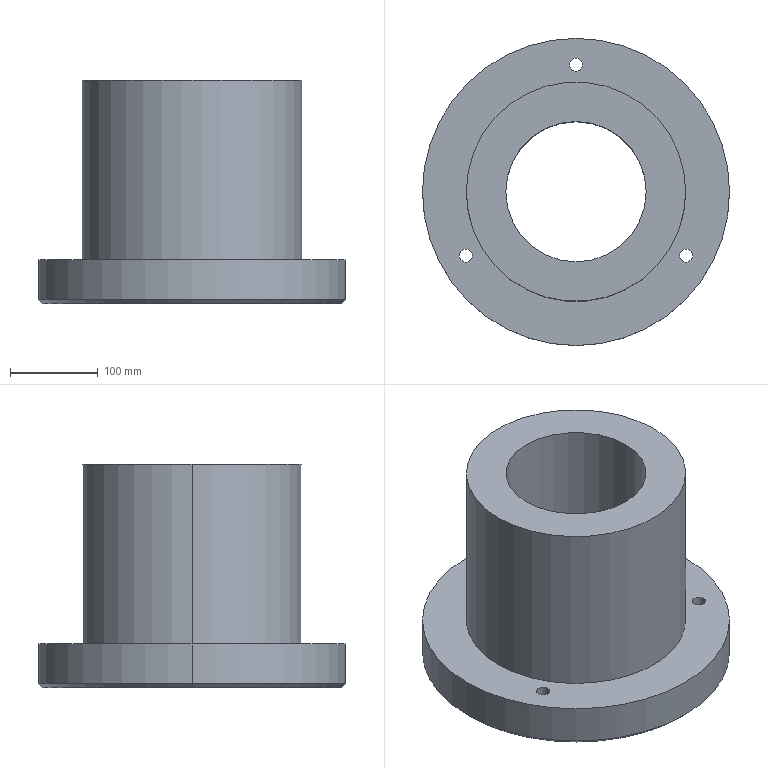Part | SolidWorks | features BaseBody 1 | 1 solid | 26 faces | box 350 x 350 x 255 mm | volume 9479362 mm3 | cylinder 14 | cone 8 | plane 4 | commonest cylinder face diameters 15 x6 160 x2 200 x2 250 x2 350 x2
STEP:
#1=CARTESIAN_POINT('',(345.077,953.249,-619.893));
#2=VERTEX_POINT('',#1);
#3=CARTESIAN_POINT('',(185.077,953.249,-619.893));
#4=VERTEX_POINT('',#3);
#5=CARTESIAN_POINT('',(265.077,953.249,-619.893));
#6=DIRECTION('',(0.,0.,-1.));
#7=DIRECTION('',(-1.,0.,0.));
#8=AXIS2_PLACEMENT_3D('',#5,#6,#7);
#9=CIRCLE('',#8,80.);
#10=EDGE_CURVE('',#2,#4,#9,.T.);
#11=ORIENTED_EDGE('',*,*,#10,.F.);
#12=CARTESIAN_POINT('',(265.077,953.249,-619.893));
#13=DIRECTION('',(0.,0.,-1.));
#14=DIRECTION('',(-1.,0.,0.));
#15=AXIS2_PLACEMENT_3D('',#12,#13,#14);
#16=CIRCLE('',#15,80.);
#17=EDGE_CURVE('',#4,#2,#16,.T.);
#18=ORIENTED_EDGE('',*,*,#17,.F.);
#19=EDGE_LOOP('',(#11,#18));
#20=FACE_BOUND('',#19,.T.);
#21=CARTESIAN_POINT('',(165.077,953.249,-619.893));
#22=VERTEX_POINT('',#21);
#23=CARTESIAN_POINT('',(365.077,953.249,-619.893));
#24=VERTEX_POINT('',#23);
#25=CARTESIAN_POINT('',(265.077,953.249,-619.893));
#26=DIRECTION('',(0.,0.,-1.));
#27=DIRECTION('',(-1.,0.,0.));
#28=AXIS2_PLACEMENT_3D('',#25,#26,#27);
#29=CIRCLE('',#28,100.);
#30=EDGE_CURVE('',#22,#24,#29,.T.);
#31=ORIENTED_EDGE('',*,*,#30,.T.);
#32=CARTESIAN_POINT('',(265.077,953.249,-619.893));
#33=DIRECTION('',(0.,0.,-1.));
#34=DIRECTION('',(-1.,0.,0.));
#35=AXIS2_PLACEMENT_3D('',#32,#33,#34);
#36=CIRCLE('',#35,100.);
#37=EDGE_CURVE('',#24,#22,#36,.T.);
#38=ORIENTED_EDGE('',*,*,#37,.T.);
#39=EDGE_LOOP('',(#31,#38));
#40=FACE_OUTER_BOUND('',#39,.T.);
#41=CARTESIAN_POINT('',(265.077,953.249,-619.893));
#42=DIRECTION('',(0.,0.,-1.));
#43=DIRECTION('',(0.,-1.,0.));
#44=AXIS2_PLACEMENT_3D('',#41,#42,#43);
#45=PLANE('',#44);
#46=ADVANCED_FACE('',(#20,#40),#45,.T.);
#47=CARTESIAN_POINT('',(365.077,953.249,-639.893));
#48=VERTEX_POINT('',#47);
#49=CARTESIAN_POINT('',(365.077,953.249,-619.893));
#50=DIRECTION('',(0.,0.,1.));
#51=VECTOR('',#50,1000.);
#52=LINE('',#49,#51);
#53=EDGE_CURVE('',#48,#24,#52,.T.);
#54=ORIENTED_EDGE('',*,*,#53,.T.);
#55=ORIENTED_EDGE('',*,*,#30,.F.);
#56=CARTESIAN_POINT('',(165.077,953.249,-639.893));
#57=VERTEX_POINT('',#56);
#58=CARTESIAN_POINT('',(165.077,953.249,-619.893));
#59=DIRECTION('',(0.,0.,1.));
#60=VECTOR('',#59,1000.);
#61=LINE('',#58,#60);
#62=EDGE_CURVE('',#57,#22,#61,.T.);
#63=ORIENTED_EDGE('',*,*,#62,.F.);
#64=CARTESIAN_POINT('',(265.077,953.249,-639.893));
#65=DIRECTION('',(0.,0.,-1.));
#66=DIRECTION('',(-1.,0.,0.));
#67=AXIS2_PLACEMENT_3D('',#64,#65,#66);
#68=CIRCLE('',#67,100.);
#69=EDGE_CURVE('',#57,#48,#68,.T.);
#70=ORIENTED_EDGE('',*,*,#69,.T.);
#71=EDGE_LOOP('',(#54,#55,#63,#70));
#72=FACE_OUTER_BOUND('',#71,.T.);
#73=CARTESIAN_POINT('',(265.077,953.249,-619.893));
#74=DIRECTION('',(0.,0.,-1.));
#75=DIRECTION('',(1.,0.,0.));
#76=AXIS2_PLACEMENT_3D('',#73,#74,#75);
#77=CYLINDRICAL_SURFACE('',#76,100.);
#78=ADVANCED_FACE('',(#72),#77,.F.);
#79=CARTESIAN_POINT('',(90.077,953.249,-634.893));
#80=VERTEX_POINT('',#79);
#81=CARTESIAN_POINT('',(95.077,953.249,-639.893));
#82=VERTEX_POINT('',#81);
#83=CARTESIAN_POINT('',(95.077,953.249,-639.893));
#84=DIRECTION('',(0.7071,0.,-0.7071));
#85=VECTOR('',#84,1000.);
#86=LINE('',#83,#85);
#87=EDGE_CURVE('',#80,#82,#86,.T.);
#88=ORIENTED_EDGE('',*,*,#87,.T.);
#89=CARTESIAN_POINT('',(435.077,953.249,-639.893));
#90=VERTEX_POINT('',#89);
#91=CARTESIAN_POINT('',(265.077,953.249,-639.893));
#92=DIRECTION('',(0.,0.,-1.));
#93=DIRECTION('',(-1.,0.,0.));
#94=AXIS2_PLACEMENT_3D('',#91,#92,#93);
#95=CIRCLE('',#94,170.);
#96=EDGE_CURVE('',#90,#82,#95,.T.);
#97=ORIENTED_EDGE('',*,*,#96,.F.);
#98=CARTESIAN_POINT('',(440.077,953.249,-634.893));
#99=VERTEX_POINT('',#98);
#100=CARTESIAN_POINT('',(435.077,953.249,-639.893));
#101=DIRECTION('',(-0.7071,0.,-0.7071));
#102=VECTOR('',#101,1000.);
#103=LINE('',#100,#102);
#104=EDGE_CURVE('',#99,#90,#103,.T.);
#105=ORIENTED_EDGE('',*,*,#104,.F.);
#106=CARTESIAN_POINT('',(265.077,953.249,-634.893));
#107=DIRECTION('',(0.,0.,1.));
#108=DIRECTION('',(-1.,0.,0.));
#109=AXIS2_PLACEMENT_3D('',#106,#107,#108);
#110=CIRCLE('',#109,175.);
#111=EDGE_CURVE('',#80,#99,#110,.T.);
#112=ORIENTED_EDGE('',*,*,#111,.F.);
#113=EDGE_LOOP('',(#88,#97,#105,#112));
#114=FACE_OUTER_BOUND('',#113,.T.);
#115=CARTESIAN_POINT('',(265.077,953.249,-639.893));
#116=DIRECTION('',(0.,0.,1.));
#117=DIRECTION('',(-1.,0.,0.));
#118=AXIS2_PLACEMENT_3D('',#115,#116,#117);
#119=CONICAL_SURFACE('',#118,170.,0.7854);
#120=ADVANCED_FACE('',(#114),#119,.T.);
#121=CARTESIAN_POINT('',(275.577,1098.249,-639.893));
#122=VERTEX_POINT('',#121);
#123=CARTESIAN_POINT('',(272.577,1098.249,-636.893));
#124=VERTEX_POINT('',#123);
#125=CARTESIAN_POINT('',(272.577,1098.249,-636.893));
#126=DIRECTION('',(-0.7071,0.,0.7071));
#127=VECTOR('',#126,1000.);
#128=LINE('',#125,#127);
#129=EDGE_CURVE('',#122,#124,#128,.T.);
#130=ORIENTED_EDGE('',*,*,#129,.T.);
#131=CARTESIAN_POINT('',(257.577,1098.249,-636.893));
#132=VERTEX_POINT('',#131);
#133=CARTESIAN_POINT('',(265.077,1098.249,-636.893));
#134=DIRECTION('',(0.,0.,-1.));
#135=DIRECTION('',(-1.,0.,0.));
#136=AXIS2_PLACEMENT_3D('',#133,#134,#135);
#137=CIRCLE('',#136,7.5);
#138=EDGE_CURVE('',#132,#124,#137,.T.);
#139=ORIENTED_EDGE('',*,*,#138,.F.);
#140=CARTESIAN_POINT('',(254.577,1098.249,-639.893));
#141=VERTEX_POINT('',#140);
#142=CARTESIAN_POINT('',(257.577,1098.249,-636.893));
#143=DIRECTION('',(0.7071,0.,0.7071));
#144=VECTOR('',#143,1000.);
#145=LINE('',#142,#144);
#146=EDGE_CURVE('',#141,#132,#145,.T.);
#147=ORIENTED_EDGE('',*,*,#146,.F.);
#148=CARTESIAN_POINT('',(265.077,1098.249,-639.893));
#149=DIRECTION('',(0.,0.,1.));
#150=DIRECTION('',(-1.,0.,0.));
#151=AXIS2_PLACEMENT_3D('',#148,#149,#150);
#152=CIRCLE('',#151,10.5);
#153=EDGE_CURVE('',#122,#141,#152,.T.);
#154=ORIENTED_EDGE('',*,*,#153,.F.);
#155=EDGE_LOOP('',(#130,#139,#147,#154));
#156=FACE_OUTER_BOUND('',#155,.T.);
#157=CARTESIAN_POINT('',(265.077,1098.249,-636.893));
#158=DIRECTION('',(0.,0.,-1.));
#159=DIRECTION('',(1.,0.,0.));
#160=AXIS2_PLACEMENT_3D('',#157,#158,#159);
#161=CONICAL_SURFACE('',#160,7.5,0.7854);
#162=ADVANCED_FACE('',(#156),#161,.F.);
#163=CARTESIAN_POINT('',(401.151,880.749,-639.893));
#164=VERTEX_POINT('',#163);
#165=CARTESIAN_POINT('',(398.151,880.749,-636.893));
#166=VERTEX_POINT('',#165);
#167=CARTESIAN_POINT('',(398.151,880.749,-636.893));
#168=DIRECTION('',(-0.7071,0.,0.7071));
#169=VECTOR('',#168,1000.);
#170=LINE('',#167,#169);
#171=EDGE_CURVE('',#164,#166,#170,.T.);
#172=ORIENTED_EDGE('',*,*,#171,.T.);
#173=CARTESIAN_POINT('',(383.151,880.749,-636.893));
#174=VERTEX_POINT('',#173);
#175=CARTESIAN_POINT('',(390.651,880.749,-636.893));
#176=DIRECTION('',(0.,0.,-1.));
#177=DIRECTION('',(-1.,0.,0.));
#178=AXIS2_PLACEMENT_3D('',#175,#176,#177);
#179=CIRCLE('',#178,7.5);
#180=EDGE_CURVE('',#174,#166,#179,.T.);
#181=ORIENTED_EDGE('',*,*,#180,.F.);
#182=CARTESIAN_POINT('',(380.151,880.749,-639.893));
#183=VERTEX_POINT('',#182);
#184=CARTESIAN_POINT('',(383.151,880.749,-636.893));
#185=DIRECTION('',(0.7071,0.,0.7071));
#186=VECTOR('',#185,1000.);
#187=LINE('',#184,#186);
#188=EDGE_CURVE('',#183,#174,#187,.T.);
#189=ORIENTED_EDGE('',*,*,#188,.F.);
#190=CARTESIAN_POINT('',(390.651,880.749,-639.893));
#191=DIRECTION('',(0.,0.,1.));
#192=DIRECTION('',(-1.,0.,0.));
#193=AXIS2_PLACEMENT_3D('',#190,#191,#192);
#194=CIRCLE('',#193,10.5);
#195=EDGE_CURVE('',#164,#183,#194,.T.);
#196=ORIENTED_EDGE('',*,*,#195,.F.);
#197=EDGE_LOOP('',(#172,#181,#189,#196));
#198=FACE_OUTER_BOUND('',#197,.T.);
#199=CARTESIAN_POINT('',(390.651,880.749,-636.893));
#200=DIRECTION('',(0.,0.,-1.));
#201=DIRECTION('',(1.,0.,0.));
#202=AXIS2_PLACEMENT_3D('',#199,#200,#201);
#203=CONICAL_SURFACE('',#202,7.5,0.7854);
#204=ADVANCED_FACE('',(#198),#203,.F.);
#205=CARTESIAN_POINT('',(150.003,880.749,-639.893));
#206=VERTEX_POINT('',#205);
#207=CARTESIAN_POINT('',(147.003,880.749,-636.893));
#208=VERTEX_POINT('',#207);
#209=CARTESIAN_POINT('',(147.003,880.749,-636.893));
#210=DIRECTION('',(-0.7071,0.,0.7071));
#211=VECTOR('',#210,1000.);
#212=LINE('',#209,#211);
#213=EDGE_CURVE('',#206,#208,#212,.T.);
#214=ORIENTED_EDGE('',*,*,#213,.T.);
#215=CARTESIAN_POINT('',(132.003,880.749,-636.893));
#216=VERTEX_POINT('',#215);
#217=CARTESIAN_POINT('',(139.503,880.749,-636.893));
#218=DIRECTION('',(0.,0.,-1.));
#219=DIRECTION('',(-1.,0.,0.));
#220=AXIS2_PLACEMENT_3D('',#217,#218,#219);
#221=CIRCLE('',#220,7.5);
#222=EDGE_CURVE('',#216,#208,#221,.T.);
#223=ORIENTED_EDGE('',*,*,#222,.F.);
#224=CARTESIAN_POINT('',(129.003,880.749,-639.893));
#225=VERTEX_POINT('',#224);
#226=CARTESIAN_POINT('',(132.003,880.749,-636.893));
#227=DIRECTION('',(0.7071,0.,0.7071));
#228=VECTOR('',#227,1000.);
#229=LINE('',#226,#228);
#230=EDGE_CURVE('',#225,#216,#229,.T.);
#231=ORIENTED_EDGE('',*,*,#230,.F.);
#232=CARTESIAN_POINT('',(139.503,880.749,-639.893));
#233=DIRECTION('',(0.,0.,1.));
#234=DIRECTION('',(-1.,0.,0.));
#235=AXIS2_PLACEMENT_3D('',#232,#233,#234);
#236=CIRCLE('',#235,10.5);
#237=EDGE_CURVE('',#206,#225,#236,.T.);
#238=ORIENTED_EDGE('',*,*,#237,.F.);
#239=EDGE_LOOP('',(#214,#223,#231,#238));
#240=FACE_OUTER_BOUND('',#239,.T.);
#241=CARTESIAN_POINT('',(139.503,880.749,-636.893));
#242=DIRECTION('',(0.,0.,-1.));
#243=DIRECTION('',(1.,0.,0.));
#244=AXIS2_PLACEMENT_3D('',#241,#242,#243);
#245=CONICAL_SURFACE('',#244,7.5,0.7854);
#246=ADVANCED_FACE('',(#240),#245,.F.);
#247=CARTESIAN_POINT('',(398.151,880.749,-589.893));
#248=VERTEX_POINT('',#247);
#249=CARTESIAN_POINT('',(398.151,880.749,-568.68));
#250=DIRECTION('',(0.,0.,1.));
#251=VECTOR('',#250,1000.);
#252=LINE('',#249,#251);
#253=EDGE_CURVE('',#166,#248,#252,.T.);
#254=ORIENTED_EDGE('',*,*,#253,.T.);
#255=CARTESIAN_POINT('',(383.151,880.749,-589.893));
#256=VERTEX_POINT('',#255);
#257=CARTESIAN_POINT('',(390.651,880.749,-589.893));
#258=DIRECTION('',(0.,0.,1.));
#259=DIRECTION('',(-1.,0.,0.));
#260=AXIS2_PLACEMENT_3D('',#257,#258,#259);
#261=CIRCLE('',#260,7.5);
#262=EDGE_CURVE('',#248,#256,#261,.T.);
#263=ORIENTED_EDGE('',*,*,#262,.T.);
#264=CARTESIAN_POINT('',(383.151,880.749,-568.68));
#265=DIRECTION('',(0.,0.,1.));
#266=VECTOR('',#265,1000.);
#267=LINE('',#264,#266);
#268=EDGE_CURVE('',#174,#256,#267,.T.);
#269=ORIENTED_EDGE('',*,*,#268,.F.);
#270=ORIENTED_EDGE('',*,*,#180,.T.);
#271=EDGE_LOOP('',(#254,#263,#269,#270));
#272=FACE_OUTER_BOUND('',#271,.T.);
#273=CARTESIAN_POINT('',(390.651,880.749,-568.68));
#274=DIRECTION('',(0.,0.,-1.));
#275=DIRECTION('',(1.,0.,0.));
#276=AXIS2_PLACEMENT_3D('',#273,#274,#275);
#277=CYLINDRICAL_SURFACE('',#276,7.5);
#278=ADVANCED_FACE('',(#272),#277,.F.);
#279=CARTESIAN_POINT('',(147.003,880.749,-589.893));
#280=VERTEX_POINT('',#279);
#281=CARTESIAN_POINT('',(147.003,880.749,-568.68));
#282=DIRECTION('',(0.,0.,1.));
#283=VECTOR('',#282,1000.);
#284=LINE('',#281,#283);
#285=EDGE_CURVE('',#208,#280,#284,.T.);
#286=ORIENTED_EDGE('',*,*,#285,.T.);
#287=CARTESIAN_POINT('',(132.003,880.749,-589.893));
#288=VERTEX_POINT('',#287);
#289=CARTESIAN_POINT('',(139.503,880.749,-589.893));
#290=DIRECTION('',(0.,0.,1.));
#291=DIRECTION('',(-1.,0.,0.));
#292=AXIS2_PLACEMENT_3D('',#289,#290,#291);
#293=CIRCLE('',#292,7.5);
#294=EDGE_CURVE('',#280,#288,#293,.T.);
#295=ORIENTED_EDGE('',*,*,#294,.T.);
#296=CARTESIAN_POINT('',(132.003,880.749,-568.68));
#297=DIRECTION('',(0.,0.,1.));
#298=VECTOR('',#297,1000.);
#299=LINE('',#296,#298);
#300=EDGE_CURVE('',#216,#288,#299,.T.);
#301=ORIENTED_EDGE('',*,*,#300,.F.);
#302=ORIENTED_EDGE('',*,*,#222,.T.);
#303=EDGE_LOOP('',(#286,#295,#301,#302));
#304=FACE_OUTER_BOUND('',#303,.T.);
#305=CARTESIAN_POINT('',(139.503,880.749,-568.68));
#306=DIRECTION('',(0.,0.,-1.));
#307=DIRECTION('',(1.,0.,0.));
#308=AXIS2_PLACEMENT_3D('',#305,#306,#307);
#309=CYLINDRICAL_SURFACE('',#308,7.5);
#310=ADVANCED_FACE('',(#304),#309,.F.);
#311=CARTESIAN_POINT('',(272.577,1098.249,-589.893));
#312=VERTEX_POINT('',#311);
#313=CARTESIAN_POINT('',(272.577,1098.249,-568.68));
#314=DIRECTION('',(0.,0.,1.));
#315=VECTOR('',#314,1000.);
#316=LINE('',#313,#315);
#317=EDGE_CURVE('',#124,#312,#316,.T.);
#318=ORIENTED_EDGE('',*,*,#317,.T.);
#319=CARTESIAN_POINT('',(257.577,1098.249,-589.893));
#320=VERTEX_POINT('',#319);
#321=CARTESIAN_POINT('',(265.077,1098.249,-589.893));
#322=DIRECTION('',(0.,0.,1.));
#323=DIRECTION('',(-1.,0.,0.));
#324=AXIS2_PLACEMENT_3D('',#321,#322,#323);
#325=CIRCLE('',#324,7.5);
#326=EDGE_CURVE('',#312,#320,#325,.T.);
#327=ORIENTED_EDGE('',*,*,#326,.T.);
#328=CARTESIAN_POINT('',(257.577,1098.249,-568.68));
#329=DIRECTION('',(0.,0.,1.));
#330=VECTOR('',#329,1000.);
#331=LINE('',#328,#330);
#332=EDGE_CURVE('',#132,#320,#331,.T.);
#333=ORIENTED_EDGE('',*,*,#332,.F.);
#334=ORIENTED_EDGE('',*,*,#138,.T.);
#335=EDGE_LOOP('',(#318,#327,#333,#334));
#336=FACE_OUTER_BOUND('',#335,.T.);
#337=CARTESIAN_POINT('',(265.077,1098.249,-568.68));
#338=DIRECTION('',(0.,0.,-1.));
#339=DIRECTION('',(1.,0.,0.));
#340=AXIS2_PLACEMENT_3D('',#337,#338,#339);
#341=CYLINDRICAL_SURFACE('',#340,7.5);
#342=ADVANCED_FACE('',(#336),#341,.F.);
#343=CARTESIAN_POINT('',(265.077,1098.249,-639.893));
#344=DIRECTION('',(0.,0.,1.));
#345=DIRECTION('',(-1.,0.,0.));
#346=AXIS2_PLACEMENT_3D('',#343,#344,#345);
#347=CIRCLE('',#346,10.5);
#348=EDGE_CURVE('',#141,#122,#347,.T.);
#349=ORIENTED_EDGE('',*,*,#348,.T.);
#350=ORIENTED_EDGE('',*,*,#153,.T.);
#351=EDGE_LOOP('',(#349,#350));
#352=FACE_BOUND('',#351,.T.);
#353=CARTESIAN_POINT('',(390.651,880.749,-639.893));
#354=DIRECTION('',(0.,0.,1.));
#355=DIRECTION('',(-1.,0.,0.));
#356=AXIS2_PLACEMENT_3D('',#353,#354,#355);
#357=CIRCLE('',#356,10.5);
#358=EDGE_CURVE('',#183,#164,#357,.T.);
#359=ORIENTED_EDGE('',*,*,#358,.T.);
#360=ORIENTED_EDGE('',*,*,#195,.T.);
#361=EDGE_LOOP('',(#359,#360));
#362=FACE_BOUND('',#361,.T.);
#363=CARTESIAN_POINT('',(139.503,880.749,-639.893));
#364=DIRECTION('',(0.,0.,1.));
#365=DIRECTION('',(-1.,0.,0.));
#366=AXIS2_PLACEMENT_3D('',#363,#364,#365);
#367=CIRCLE('',#366,10.5);
#368=EDGE_CURVE('',#225,#206,#367,.T.);
#369=ORIENTED_EDGE('',*,*,#368,.T.);
#370=ORIENTED_EDGE('',*,*,#237,.T.);
#371=EDGE_LOOP('',(#369,#370));
#372=FACE_BOUND('',#371,.T.);
#373=ORIENTED_EDGE('',*,*,#69,.F.);
#374=CARTESIAN_POINT('',(265.077,953.249,-639.893));
#375=DIRECTION('',(0.,0.,-1.));
#376=DIRECTION('',(-1.,0.,0.));
#377=AXIS2_PLACEMENT_3D('',#374,#375,#376);
#378=CIRCLE('',#377,100.);
#379=EDGE_CURVE('',#48,#57,#378,.T.);
#380=ORIENTED_EDGE('',*,*,#379,.F.);
#381=EDGE_LOOP('',(#373,#380));
#382=FACE_BOUND('',#381,.T.);
#383=ORIENTED_EDGE('',*,*,#96,.T.);
#384=CARTESIAN_POINT('',(265.077,953.249,-639.893));
#385=DIRECTION('',(0.,0.,-1.));
#386=DIRECTION('',(-1.,0.,0.));
#387=AXIS2_PLACEMENT_3D('',#384,#385,#386);
#388=CIRCLE('',#387,170.);
#389=EDGE_CURVE('',#82,#90,#388,.T.);
#390=ORIENTED_EDGE('',*,*,#389,.T.);
#391=EDGE_LOOP('',(#383,#390));
#392=FACE_OUTER_BOUND('',#391,.T.);
#393=CARTESIAN_POINT('',(265.077,953.249,-639.893));
#394=DIRECTION('',(0.,0.,-1.));
#395=DIRECTION('',(0.,-1.,0.));
#396=AXIS2_PLACEMENT_3D('',#393,#394,#395);
#397=PLANE('',#396);
#398=ADVANCED_FACE('',(#352,#362,#372,#382,#392),#397,.T.);
#399=CARTESIAN_POINT('',(90.077,953.249,-589.893));
#400=VERTEX_POINT('',#399);
#401=CARTESIAN_POINT('',(90.077,953.249,-639.893));
#402=DIRECTION('',(0.,0.,-1.));
#403=VECTOR('',#402,1000.);
#404=LINE('',#401,#403);
#405=EDGE_CURVE('',#400,#80,#404,.T.);
#406=ORIENTED_EDGE('',*,*,#405,.T.);
#407=ORIENTED_EDGE('',*,*,#111,.T.);
#408=CARTESIAN_POINT('',(440.077,953.249,-589.893));
#409=VERTEX_POINT('',#408);
#410=CARTESIAN_POINT('',(440.077,953.249,-639.893));
#411=DIRECTION('',(0.,0.,-1.));
#412=VECTOR('',#411,1000.);
#413=LINE('',#410,#412);
#414=EDGE_CURVE('',#409,#99,#413,.T.);
#415=ORIENTED_EDGE('',*,*,#414,.F.);
#416=CARTESIAN_POINT('',(265.077,953.249,-589.893));
#417=DIRECTION('',(0.,0.,-1.));
#418=DIRECTION('',(-1.,0.,0.));
#419=AXIS2_PLACEMENT_3D('',#416,#417,#418);
#420=CIRCLE('',#419,175.);
#421=EDGE_CURVE('',#409,#400,#420,.T.);
#422=ORIENTED_EDGE('',*,*,#421,.T.);
#423=EDGE_LOOP('',(#406,#407,#415,#422));
#424=FACE_OUTER_BOUND('',#423,.T.);
#425=CARTESIAN_POINT('',(265.077,953.249,-639.893));
#426=DIRECTION('',(0.,0.,1.));
#427=DIRECTION('',(-1.,0.,0.));
#428=AXIS2_PLACEMENT_3D('',#425,#426,#427);
#429=CYLINDRICAL_SURFACE('',#428,175.);
#430=ADVANCED_FACE('',(#424),#429,.T.);
#431=CARTESIAN_POINT('',(390.077,953.249,-589.893));
#432=VERTEX_POINT('',#431);
#433=CARTESIAN_POINT('',(140.077,953.249,-589.893));
#434=VERTEX_POINT('',#433);
#435=CARTESIAN_POINT('',(265.077,953.249,-589.893));
#436=DIRECTION('',(0.,0.,-1.));
#437=DIRECTION('',(-1.,0.,0.));
#438=AXIS2_PLACEMENT_3D('',#435,#436,#437);
#439=CIRCLE('',#438,125.);
#440=EDGE_CURVE('',#432,#434,#439,.T.);
#441=ORIENTED_EDGE('',*,*,#440,.T.);
#442=CARTESIAN_POINT('',(265.077,953.249,-589.893));
#443=DIRECTION('',(0.,0.,-1.));
#444=DIRECTION('',(-1.,0.,0.));
#445=AXIS2_PLACEMENT_3D('',#442,#443,#444);
#446=CIRCLE('',#445,125.);
#447=EDGE_CURVE('',#434,#432,#446,.T.);
#448=ORIENTED_EDGE('',*,*,#447,.T.);
#449=EDGE_LOOP('',(#441,#448));
#450=FACE_BOUND('',#449,.T.);
#451=CARTESIAN_POINT('',(265.077,1098.249,-589.893));
#452=DIRECTION('',(0.,0.,1.));
#453=DIRECTION('',(-1.,0.,0.));
#454=AXIS2_PLACEMENT_3D('',#451,#452,#453);
#455=CIRCLE('',#454,7.5);
#456=EDGE_CURVE('',#320,#312,#455,.T.);
#457=ORIENTED_EDGE('',*,*,#456,.F.);
#458=ORIENTED_EDGE('',*,*,#326,.F.);
#459=EDGE_LOOP('',(#457,#458));
#460=FACE_BOUND('',#459,.T.);
#461=CARTESIAN_POINT('',(139.503,880.749,-589.893));
#462=DIRECTION('',(0.,0.,1.));
#463=DIRECTION('',(-1.,0.,0.));
#464=AXIS2_PLACEMENT_3D('',#461,#462,#463);
#465=CIRCLE('',#464,7.5);
#466=EDGE_CURVE('',#288,#280,#465,.T.);
#467=ORIENTED_EDGE('',*,*,#466,.F.);
#468=ORIENTED_EDGE('',*,*,#294,.F.);
#469=EDGE_LOOP('',(#467,#468));
#470=FACE_BOUND('',#469,.T.);
#471=CARTESIAN_POINT('',(390.651,880.749,-589.893));
#472=DIRECTION('',(0.,0.,1.));
#473=DIRECTION('',(-1.,0.,0.));
#474=AXIS2_PLACEMENT_3D('',#471,#472,#473);
#475=CIRCLE('',#474,7.5);
#476=EDGE_CURVE('',#256,#248,#475,.T.);
#477=ORIENTED_EDGE('',*,*,#476,.F.);
#478=ORIENTED_EDGE('',*,*,#262,.F.);
#479=EDGE_LOOP('',(#477,#478));
#480=FACE_BOUND('',#479,.T.);
#481=ORIENTED_EDGE('',*,*,#421,.F.);
#482=CARTESIAN_POINT('',(265.077,953.249,-589.893));
#483=DIRECTION('',(0.,0.,-1.));
#484=DIRECTION('',(-1.,0.,0.));
#485=AXIS2_PLACEMENT_3D('',#482,#483,#484);
#486=CIRCLE('',#485,175.);
#487=EDGE_CURVE('',#400,#409,#486,.T.);
#488=ORIENTED_EDGE('',*,*,#487,.F.);
#489=EDGE_LOOP('',(#481,#488));
#490=FACE_OUTER_BOUND('',#489,.T.);
#491=CARTESIAN_POINT('',(265.077,953.249,-589.893));
#492=DIRECTION('',(0.,0.,-1.));
#493=DIRECTION('',(0.,-1.,0.));
#494=AXIS2_PLACEMENT_3D('',#491,#492,#493);
#495=PLANE('',#494);
#496=ADVANCED_FACE('',(#450,#460,#470,#480,#490),#495,.F.);
#497=CARTESIAN_POINT('',(140.077,953.249,-384.893));
#498=VERTEX_POINT('',#497);
#499=CARTESIAN_POINT('',(140.077,953.249,-589.893));
#500=DIRECTION('',(0.,0.,-1.));
#501=VECTOR('',#500,1000.);
#502=LINE('',#499,#501);
#503=EDGE_CURVE('',#498,#434,#502,.T.);
#504=ORIENTED_EDGE('',*,*,#503,.T.);
#505=ORIENTED_EDGE('',*,*,#440,.F.);
#506=CARTESIAN_POINT('',(390.077,953.249,-384.893));
#507=VERTEX_POINT('',#506);
#508=CARTESIAN_POINT('',(390.077,953.249,-589.893));
#509=DIRECTION('',(0.,0.,-1.));
#510=VECTOR('',#509,1000.);
#511=LINE('',#508,#510);
#512=EDGE_CURVE('',#507,#432,#511,.T.);
#513=ORIENTED_EDGE('',*,*,#512,.F.);
#514=CARTESIAN_POINT('',(265.077,953.249,-384.893));
#515=DIRECTION('',(0.,0.,-1.));
#516=DIRECTION('',(-1.,0.,0.));
#517=AXIS2_PLACEMENT_3D('',#514,#515,#516);
#518=CIRCLE('',#517,125.);
#519=EDGE_CURVE('',#507,#498,#518,.T.);
#520=ORIENTED_EDGE('',*,*,#519,.T.);
#521=EDGE_LOOP('',(#504,#505,#513,#520));
#522=FACE_OUTER_BOUND('',#521,.T.);
#523=CARTESIAN_POINT('',(265.077,953.249,-589.893));
#524=DIRECTION('',(0.,0.,1.));
#525=DIRECTION('',(-1.,0.,0.));
#526=AXIS2_PLACEMENT_3D('',#523,#524,#525);
#527=CYLINDRICAL_SURFACE('',#526,125.);
#528=ADVANCED_FACE('',(#522),#527,.T.);
#529=CARTESIAN_POINT('',(345.077,953.249,-384.893));
#530=VERTEX_POINT('',#529);
#531=CARTESIAN_POINT('',(185.077,953.249,-384.893));
#532=VERTEX_POINT('',#531);
#533=CARTESIAN_POINT('',(265.077,953.249,-384.893));
#534=DIRECTION('',(0.,0.,-1.));
#535=DIRECTION('',(-1.,0.,0.));
#536=AXIS2_PLACEMENT_3D('',#533,#534,#535);
#537=CIRCLE('',#536,80.);
#538=EDGE_CURVE('',#530,#532,#537,.T.);
#539=ORIENTED_EDGE('',*,*,#538,.T.);
#540=CARTESIAN_POINT('',(265.077,953.249,-384.893));
#541=DIRECTION('',(0.,0.,-1.));
#542=DIRECTION('',(-1.,0.,0.));
#543=AXIS2_PLACEMENT_3D('',#540,#541,#542);
#544=CIRCLE('',#543,80.);
#545=EDGE_CURVE('',#532,#530,#544,.T.);
#546=ORIENTED_EDGE('',*,*,#545,.T.);
#547=EDGE_LOOP('',(#539,#546));
#548=FACE_BOUND('',#547,.T.);
#549=ORIENTED_EDGE('',*,*,#519,.F.);
#550=CARTESIAN_POINT('',(265.077,953.249,-384.893));
#551=DIRECTION('',(0.,0.,-1.));
#552=DIRECTION('',(-1.,0.,0.));
#553=AXIS2_PLACEMENT_3D('',#550,#551,#552);
#554=CIRCLE('',#553,125.);
#555=EDGE_CURVE('',#498,#507,#554,.T.);
#556=ORIENTED_EDGE('',*,*,#555,.F.);
#557=EDGE_LOOP('',(#549,#556));
#558=FACE_OUTER_BOUND('',#557,.T.);
#559=CARTESIAN_POINT('',(265.077,953.249,-384.893));
#560=DIRECTION('',(0.,0.,-1.));
#561=DIRECTION('',(0.,-1.,0.));
#562=AXIS2_PLACEMENT_3D('',#559,#560,#561);
#563=PLANE('',#562);
#564=ADVANCED_FACE('',(#548,#558),#563,.F.);
#565=CARTESIAN_POINT('',(185.077,953.249,-589.893));
#566=DIRECTION('',(0.,0.,-1.));
#567=VECTOR('',#566,1000.);
#568=LINE('',#565,#567);
#569=EDGE_CURVE('',#532,#4,#568,.T.);
#570=ORIENTED_EDGE('',*,*,#569,.T.);
#571=ORIENTED_EDGE('',*,*,#17,.T.);
#572=CARTESIAN_POINT('',(345.077,953.249,-589.893));
#573=DIRECTION('',(0.,0.,-1.));
#574=VECTOR('',#573,1000.);
#575=LINE('',#572,#574);
#576=EDGE_CURVE('',#530,#2,#575,.T.);
#577=ORIENTED_EDGE('',*,*,#576,.F.);
#578=ORIENTED_EDGE('',*,*,#545,.F.);
#579=EDGE_LOOP('',(#570,#571,#577,#578));
#580=FACE_OUTER_BOUND('',#579,.T.);
#581=CARTESIAN_POINT('',(265.077,953.249,-589.893));
#582=DIRECTION('',(0.,0.,1.));
#583=DIRECTION('',(-1.,0.,0.));
#584=AXIS2_PLACEMENT_3D('',#581,#582,#583);
#585=CYLINDRICAL_SURFACE('',#584,80.);
#586=ADVANCED_FACE('',(#580),#585,.F.);
#587=ORIENTED_EDGE('',*,*,#10,.T.);
#588=ORIENTED_EDGE('',*,*,#569,.F.);
#589=ORIENTED_EDGE('',*,*,#538,.F.);
#590=ORIENTED_EDGE('',*,*,#576,.T.);
#591=EDGE_LOOP('',(#587,#588,#589,#590));
#592=FACE_OUTER_BOUND('',#591,.T.);
#593=CARTESIAN_POINT('',(265.077,953.249,-589.893));
#594=DIRECTION('',(0.,0.,1.));
#595=DIRECTION('',(-1.,0.,0.));
#596=AXIS2_PLACEMENT_3D('',#593,#594,#595);
#597=CYLINDRICAL_SURFACE('',#596,80.);
#598=ADVANCED_FACE('',(#592),#597,.F.);
#599=ORIENTED_EDGE('',*,*,#447,.F.);
#600=ORIENTED_EDGE('',*,*,#503,.F.);
#601=ORIENTED_EDGE('',*,*,#555,.T.);
#602=ORIENTED_EDGE('',*,*,#512,.T.);
#603=EDGE_LOOP('',(#599,#600,#601,#602));
#604=FACE_OUTER_BOUND('',#603,.T.);
#605=CARTESIAN_POINT('',(265.077,953.249,-589.893));
#606=DIRECTION('',(0.,0.,1.));
#607=DIRECTION('',(-1.,0.,0.));
#608=AXIS2_PLACEMENT_3D('',#605,#606,#607);
#609=CYLINDRICAL_SURFACE('',#608,125.);
#610=ADVANCED_FACE('',(#604),#609,.T.);
#611=CARTESIAN_POINT('',(265.077,953.249,-634.893));
#612=DIRECTION('',(0.,0.,1.));
#613=DIRECTION('',(-1.,0.,0.));
#614=AXIS2_PLACEMENT_3D('',#611,#612,#613);
#615=CIRCLE('',#614,175.);
#616=EDGE_CURVE('',#99,#80,#615,.T.);
#617=ORIENTED_EDGE('',*,*,#616,.T.);
#618=ORIENTED_EDGE('',*,*,#405,.F.);
#619=ORIENTED_EDGE('',*,*,#487,.T.);
#620=ORIENTED_EDGE('',*,*,#414,.T.);
#621=EDGE_LOOP('',(#617,#618,#619,#620));
#622=FACE_OUTER_BOUND('',#621,.T.);
#623=CARTESIAN_POINT('',(265.077,953.249,-639.893));
#624=DIRECTION('',(0.,0.,1.));
#625=DIRECTION('',(-1.,0.,0.));
#626=AXIS2_PLACEMENT_3D('',#623,#624,#625);
#627=CYLINDRICAL_SURFACE('',#626,175.);
#628=ADVANCED_FACE('',(#622),#627,.T.);
#629=ORIENTED_EDGE('',*,*,#456,.T.);
#630=ORIENTED_EDGE('',*,*,#317,.F.);
#631=CARTESIAN_POINT('',(265.077,1098.249,-636.893));
#632=DIRECTION('',(0.,0.,-1.));
#633=DIRECTION('',(-1.,0.,0.));
#634=AXIS2_PLACEMENT_3D('',#631,#632,#633);
#635=CIRCLE('',#634,7.5);
#636=EDGE_CURVE('',#124,#132,#635,.T.);
#637=ORIENTED_EDGE('',*,*,#636,.T.);
#638=ORIENTED_EDGE('',*,*,#332,.T.);
#639=EDGE_LOOP('',(#629,#630,#637,#638));
#640=FACE_OUTER_BOUND('',#639,.T.);
#641=CARTESIAN_POINT('',(265.077,1098.249,-568.68));
#642=DIRECTION('',(0.,0.,-1.));
#643=DIRECTION('',(1.,0.,0.));
#644=AXIS2_PLACEMENT_3D('',#641,#642,#643);
#645=CYLINDRICAL_SURFACE('',#644,7.5);
#646=ADVANCED_FACE('',(#640),#645,.F.);
#647=ORIENTED_EDGE('',*,*,#466,.T.);
#648=ORIENTED_EDGE('',*,*,#285,.F.);
#649=CARTESIAN_POINT('',(139.503,880.749,-636.893));
#650=DIRECTION('',(0.,0.,-1.));
#651=DIRECTION('',(-1.,0.,0.));
#652=AXIS2_PLACEMENT_3D('',#649,#650,#651);
#653=CIRCLE('',#652,7.5);
#654=EDGE_CURVE('',#208,#216,#653,.T.);
#655=ORIENTED_EDGE('',*,*,#654,.T.);
#656=ORIENTED_EDGE('',*,*,#300,.T.);
#657=EDGE_LOOP('',(#647,#648,#655,#656));
#658=FACE_OUTER_BOUND('',#657,.T.);
#659=CARTESIAN_POINT('',(139.503,880.749,-568.68));
#660=DIRECTION('',(0.,0.,-1.));
#661=DIRECTION('',(1.,0.,0.));
#662=AXIS2_PLACEMENT_3D('',#659,#660,#661);
#663=CYLINDRICAL_SURFACE('',#662,7.5);
#664=ADVANCED_FACE('',(#658),#663,.F.);
#665=ORIENTED_EDGE('',*,*,#476,.T.);
#666=ORIENTED_EDGE('',*,*,#253,.F.);
#667=CARTESIAN_POINT('',(390.651,880.749,-636.893));
#668=DIRECTION('',(0.,0.,-1.));
#669=DIRECTION('',(-1.,0.,0.));
#670=AXIS2_PLACEMENT_3D('',#667,#668,#669);
#671=CIRCLE('',#670,7.5);
#672=EDGE_CURVE('',#166,#174,#671,.T.);
#673=ORIENTED_EDGE('',*,*,#672,.T.);
#674=ORIENTED_EDGE('',*,*,#268,.T.);
#675=EDGE_LOOP('',(#665,#666,#673,#674));
#676=FACE_OUTER_BOUND('',#675,.T.);
#677=CARTESIAN_POINT('',(390.651,880.749,-568.68));
#678=DIRECTION('',(0.,0.,-1.));
#679=DIRECTION('',(1.,0.,0.));
#680=AXIS2_PLACEMENT_3D('',#677,#678,#679);
#681=CYLINDRICAL_SURFACE('',#680,7.5);
#682=ADVANCED_FACE('',(#676),#681,.F.);
#683=ORIENTED_EDGE('',*,*,#654,.F.);
#684=ORIENTED_EDGE('',*,*,#213,.F.);
#685=ORIENTED_EDGE('',*,*,#368,.F.);
#686=ORIENTED_EDGE('',*,*,#230,.T.);
#687=EDGE_LOOP('',(#683,#684,#685,#686));
#688=FACE_OUTER_BOUND('',#687,.T.);
#689=CARTESIAN_POINT('',(139.503,880.749,-636.893));
#690=DIRECTION('',(0.,0.,-1.));
#691=DIRECTION('',(1.,0.,0.));
#692=AXIS2_PLACEMENT_3D('',#689,#690,#691);
#693=CONICAL_SURFACE('',#692,7.5,0.7854);
#694=ADVANCED_FACE('',(#688),#693,.F.);
#695=ORIENTED_EDGE('',*,*,#672,.F.);
#696=ORIENTED_EDGE('',*,*,#171,.F.);
#697=ORIENTED_EDGE('',*,*,#358,.F.);
#698=ORIENTED_EDGE('',*,*,#188,.T.);
#699=EDGE_LOOP('',(#695,#696,#697,#698));
#700=FACE_OUTER_BOUND('',#699,.T.);
#701=CARTESIAN_POINT('',(390.651,880.749,-636.893));
#702=DIRECTION('',(0.,0.,-1.));
#703=DIRECTION('',(1.,0.,0.));
#704=AXIS2_PLACEMENT_3D('',#701,#702,#703);
#705=CONICAL_SURFACE('',#704,7.5,0.7854);
#706=ADVANCED_FACE('',(#700),#705,.F.);
#707=ORIENTED_EDGE('',*,*,#636,.F.);
#708=ORIENTED_EDGE('',*,*,#129,.F.);
#709=ORIENTED_EDGE('',*,*,#348,.F.);
#710=ORIENTED_EDGE('',*,*,#146,.T.);
#711=EDGE_LOOP('',(#707,#708,#709,#710));
#712=FACE_OUTER_BOUND('',#711,.T.);
#713=CARTESIAN_POINT('',(265.077,1098.249,-636.893));
#714=DIRECTION('',(0.,0.,-1.));
#715=DIRECTION('',(1.,0.,0.));
#716=AXIS2_PLACEMENT_3D('',#713,#714,#715);
#717=CONICAL_SURFACE('',#716,7.5,0.7854);
#718=ADVANCED_FACE('',(#712),#717,.F.);
#719=ORIENTED_EDGE('',*,*,#389,.F.);
#720=ORIENTED_EDGE('',*,*,#87,.F.);
#721=ORIENTED_EDGE('',*,*,#616,.F.);
#722=ORIENTED_EDGE('',*,*,#104,.T.);
#723=EDGE_LOOP('',(#719,#720,#721,#722));
#724=FACE_OUTER_BOUND('',#723,.T.);
#725=CARTESIAN_POINT('',(265.077,953.249,-639.893));
#726=DIRECTION('',(0.,0.,1.));
#727=DIRECTION('',(-1.,0.,0.));
#728=AXIS2_PLACEMENT_3D('',#725,#726,#727);
#729=CONICAL_SURFACE('',#728,170.,0.7854);
#730=ADVANCED_FACE('',(#724),#729,.T.);
#731=ORIENTED_EDGE('',*,*,#37,.F.);
#732=ORIENTED_EDGE('',*,*,#53,.F.);
#733=ORIENTED_EDGE('',*,*,#379,.T.);
#734=ORIENTED_EDGE('',*,*,#62,.T.);
#735=EDGE_LOOP('',(#731,#732,#733,#734));
#736=FACE_OUTER_BOUND('',#735,.T.);
#737=CARTESIAN_POINT('',(265.077,953.249,-619.893));
#738=DIRECTION('',(0.,0.,-1.));
#739=DIRECTION('',(1.,0.,0.));
#740=AXIS2_PLACEMENT_3D('',#737,#738,#739);
#741=CYLINDRICAL_SURFACE('',#740,100.);
#742=ADVANCED_FACE('',(#736),#741,.F.);
#743=CLOSED_SHELL('',(#46,#78,#120,#162,#204,#246,#278,#310,#342,#398,#430,#496,#528,#564,#586,#598,#610,#628,#646,#664,#682,#694,#706,#718,#730,#742));
#744=MANIFOLD_SOLID_BREP('',#743);
#745=CARTESIAN_POINT('',(0.,0.,0.));
#746=DIRECTION('',(0.,0.,1.));
#747=DIRECTION('',(1.,0.,0.));
#748=AXIS2_PLACEMENT_3D('',#745,#746,#747);
#749=(LENGTH_UNIT()NAMED_UNIT(*)SI_UNIT(.MILLI.,.METRE.));
#750=UNCERTAINTY_MEASURE_WITH_UNIT(LENGTH_MEASURE(0.00001),#749,'','');
#751=(NAMED_UNIT(*)PLANE_ANGLE_UNIT()SI_UNIT($,.RADIAN.));
#752=(NAMED_UNIT(*)SI_UNIT($,.STERADIAN.)SOLID_ANGLE_UNIT());
#753=(GEOMETRIC_REPRESENTATION_CONTEXT(3)GLOBAL_UNCERTAINTY_ASSIGNED_CONTEXT((#750))GLOBAL_UNIT_ASSIGNED_CONTEXT((#749,#751,#752))REPRESENTATION_CONTEXT('',''));
#754=ADVANCED_BREP_SHAPE_REPRESENTATION('',(#744,#748),#753);